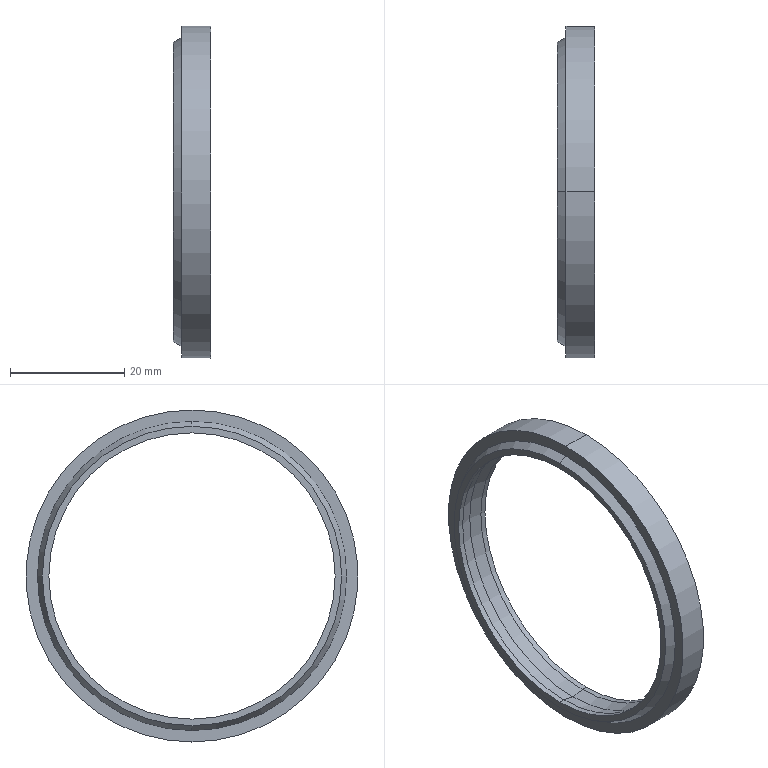Part | SolidWorks | features Revolution 2 | 1 solid | 22 faces | box 6.5 x 58 x 58 mm | volume 3242 mm3 | cone 10 | cylinder 6 | plane 4 | torus 2 | commonest cylinder face diameters 50 x4 58 x2
STEP:
#1=CARTESIAN_POINT('',(10.,0.,26.333));
#2=VERTEX_POINT('',#1);
#3=CARTESIAN_POINT('',(10.,0.,-26.333));
#4=VERTEX_POINT('',#3);
#5=CARTESIAN_POINT('',(10.,0.,0.));
#6=DIRECTION('',(-1.,0.,0.));
#7=DIRECTION('',(0.,0.,1.));
#8=AXIS2_PLACEMENT_3D('',#5,#6,#7);
#9=CIRCLE('',#8,26.333);
#10=EDGE_CURVE('',#2,#4,#9,.T.);
#11=ORIENTED_EDGE('',*,*,#10,.T.);
#12=CARTESIAN_POINT('',(7.47,0.,-26.853));
#13=VERTEX_POINT('',#12);
#14=CARTESIAN_POINT('',(10.,0.,-26.333));
#15=DIRECTION('',(-0.9795,0.,-0.2012));
#16=VECTOR('',#15,1000.);
#17=LINE('',#14,#16);
#18=EDGE_CURVE('',#4,#13,#17,.T.);
#19=ORIENTED_EDGE('',*,*,#18,.T.);
#20=CARTESIAN_POINT('',(7.47,0.,26.853));
#21=VERTEX_POINT('',#20);
#22=CARTESIAN_POINT('',(7.47,0.,0.));
#23=DIRECTION('',(-1.,0.,0.));
#24=DIRECTION('',(0.,0.,1.));
#25=AXIS2_PLACEMENT_3D('',#22,#23,#24);
#26=CIRCLE('',#25,26.853);
#27=EDGE_CURVE('',#21,#13,#26,.T.);
#28=ORIENTED_EDGE('',*,*,#27,.F.);
#29=CARTESIAN_POINT('',(10.,0.,26.333));
#30=DIRECTION('',(-0.9795,0.,0.2012));
#31=VECTOR('',#30,1000.);
#32=LINE('',#29,#31);
#33=EDGE_CURVE('',#2,#21,#32,.T.);
#34=ORIENTED_EDGE('',*,*,#33,.F.);
#35=EDGE_LOOP('',(#11,#19,#28,#34));
#36=FACE_OUTER_BOUND('',#35,.T.);
#37=CARTESIAN_POINT('',(10.,0.,0.));
#38=DIRECTION('',(-1.,0.,0.));
#39=DIRECTION('',(0.,0.,1.));
#40=AXIS2_PLACEMENT_3D('',#37,#38,#39);
#41=CONICAL_SURFACE('',#40,26.333,0.2026);
#42=ADVANCED_FACE('',(#36),#41,.T.);
#43=CARTESIAN_POINT('',(10.,0.,-25.));
#44=VERTEX_POINT('',#43);
#45=CARTESIAN_POINT('',(10.,0.,25.));
#46=VERTEX_POINT('',#45);
#47=CARTESIAN_POINT('',(10.,0.,0.));
#48=DIRECTION('',(-1.,0.,0.));
#49=DIRECTION('',(0.,0.,1.));
#50=AXIS2_PLACEMENT_3D('',#47,#48,#49);
#51=CIRCLE('',#50,25.);
#52=EDGE_CURVE('',#44,#46,#51,.T.);
#53=ORIENTED_EDGE('',*,*,#52,.F.);
#54=CARTESIAN_POINT('',(9.,0.,-25.));
#55=VERTEX_POINT('',#54);
#56=CARTESIAN_POINT('',(0.,0.,-25.));
#57=DIRECTION('',(-1.,0.,0.));
#58=VECTOR('',#57,1000.);
#59=LINE('',#56,#58);
#60=EDGE_CURVE('',#44,#55,#59,.T.);
#61=ORIENTED_EDGE('',*,*,#60,.T.);
#62=CARTESIAN_POINT('',(9.,0.,25.));
#63=VERTEX_POINT('',#62);
#64=CARTESIAN_POINT('',(9.,0.,0.));
#65=DIRECTION('',(-1.,0.,0.));
#66=DIRECTION('',(0.,0.,1.));
#67=AXIS2_PLACEMENT_3D('',#64,#65,#66);
#68=CIRCLE('',#67,25.);
#69=EDGE_CURVE('',#55,#63,#68,.T.);
#70=ORIENTED_EDGE('',*,*,#69,.T.);
#71=CARTESIAN_POINT('',(0.,0.,25.));
#72=DIRECTION('',(-1.,0.,0.));
#73=VECTOR('',#72,1000.);
#74=LINE('',#71,#73);
#75=EDGE_CURVE('',#46,#63,#74,.T.);
#76=ORIENTED_EDGE('',*,*,#75,.F.);
#77=EDGE_LOOP('',(#53,#61,#70,#76));
#78=FACE_OUTER_BOUND('',#77,.T.);
#79=CARTESIAN_POINT('',(0.,0.,0.));
#80=DIRECTION('',(-1.,0.,0.));
#81=DIRECTION('',(0.,0.,1.));
#82=AXIS2_PLACEMENT_3D('',#79,#80,#81);
#83=CYLINDRICAL_SURFACE('',#82,25.);
#84=ADVANCED_FACE('',(#78),#83,.F.);
#85=ORIENTED_EDGE('',*,*,#69,.F.);
#86=CARTESIAN_POINT('',(6.75,0.,-25.5));
#87=VERTEX_POINT('',#86);
#88=CARTESIAN_POINT('',(6.75,0.,-25.5));
#89=DIRECTION('',(-0.9762,0.,-0.2169));
#90=VECTOR('',#89,1000.);
#91=LINE('',#88,#90);
#92=EDGE_CURVE('',#55,#87,#91,.T.);
#93=ORIENTED_EDGE('',*,*,#92,.T.);
#94=CARTESIAN_POINT('',(6.75,0.,25.5));
#95=VERTEX_POINT('',#94);
#96=CARTESIAN_POINT('',(6.75,0.,0.));
#97=DIRECTION('',(-1.,0.,0.));
#98=DIRECTION('',(0.,0.,1.));
#99=AXIS2_PLACEMENT_3D('',#96,#97,#98);
#100=CIRCLE('',#99,25.5);
#101=EDGE_CURVE('',#87,#95,#100,.T.);
#102=ORIENTED_EDGE('',*,*,#101,.T.);
#103=CARTESIAN_POINT('',(6.75,0.,25.5));
#104=DIRECTION('',(-0.9762,0.,0.2169));
#105=VECTOR('',#104,1000.);
#106=LINE('',#103,#105);
#107=EDGE_CURVE('',#63,#95,#106,.T.);
#108=ORIENTED_EDGE('',*,*,#107,.F.);
#109=EDGE_LOOP('',(#85,#93,#102,#108));
#110=FACE_OUTER_BOUND('',#109,.T.);
#111=CARTESIAN_POINT('',(6.75,0.,0.));
#112=DIRECTION('',(-1.,0.,0.));
#113=DIRECTION('',(0.,0.,1.));
#114=AXIS2_PLACEMENT_3D('',#111,#112,#113);
#115=CONICAL_SURFACE('',#114,25.5,0.2187);
#116=ADVANCED_FACE('',(#110),#115,.F.);
#117=CARTESIAN_POINT('',(4.5,0.,-25.));
#118=VERTEX_POINT('',#117);
#119=CARTESIAN_POINT('',(4.5,0.,25.));
#120=VERTEX_POINT('',#119);
#121=CARTESIAN_POINT('',(4.5,0.,0.));
#122=DIRECTION('',(-1.,0.,0.));
#123=DIRECTION('',(0.,0.,1.));
#124=AXIS2_PLACEMENT_3D('',#121,#122,#123);
#125=CIRCLE('',#124,25.);
#126=EDGE_CURVE('',#118,#120,#125,.T.);
#127=ORIENTED_EDGE('',*,*,#126,.T.);
#128=CARTESIAN_POINT('',(4.5,0.,25.));
#129=DIRECTION('',(0.9762,0.,0.2169));
#130=VECTOR('',#129,1000.);
#131=LINE('',#128,#130);
#132=EDGE_CURVE('',#120,#95,#131,.T.);
#133=ORIENTED_EDGE('',*,*,#132,.T.);
#134=ORIENTED_EDGE('',*,*,#101,.F.);
#135=CARTESIAN_POINT('',(4.5,0.,-25.));
#136=DIRECTION('',(0.9762,0.,-0.2169));
#137=VECTOR('',#136,1000.);
#138=LINE('',#135,#137);
#139=EDGE_CURVE('',#118,#87,#138,.T.);
#140=ORIENTED_EDGE('',*,*,#139,.F.);
#141=EDGE_LOOP('',(#127,#133,#134,#140));
#142=FACE_OUTER_BOUND('',#141,.T.);
#143=CARTESIAN_POINT('',(4.5,0.,0.));
#144=DIRECTION('',(1.,0.,0.));
#145=DIRECTION('',(0.,0.,-1.));
#146=AXIS2_PLACEMENT_3D('',#143,#144,#145);
#147=CONICAL_SURFACE('',#146,25.,0.2187);
#148=ADVANCED_FACE('',(#142),#147,.F.);
#149=ORIENTED_EDGE('',*,*,#126,.F.);
#150=CARTESIAN_POINT('',(3.5,0.,-25.));
#151=VERTEX_POINT('',#150);
#152=CARTESIAN_POINT('',(0.,0.,-25.));
#153=DIRECTION('',(-1.,0.,0.));
#154=VECTOR('',#153,1000.);
#155=LINE('',#152,#154);
#156=EDGE_CURVE('',#118,#151,#155,.T.);
#157=ORIENTED_EDGE('',*,*,#156,.T.);
#158=CARTESIAN_POINT('',(3.5,0.,25.));
#159=VERTEX_POINT('',#158);
#160=CARTESIAN_POINT('',(3.5,0.,0.));
#161=DIRECTION('',(-1.,0.,0.));
#162=DIRECTION('',(0.,0.,1.));
#163=AXIS2_PLACEMENT_3D('',#160,#161,#162);
#164=CIRCLE('',#163,25.);
#165=EDGE_CURVE('',#151,#159,#164,.T.);
#166=ORIENTED_EDGE('',*,*,#165,.T.);
#167=CARTESIAN_POINT('',(0.,0.,25.));
#168=DIRECTION('',(-1.,0.,0.));
#169=VECTOR('',#168,1000.);
#170=LINE('',#167,#169);
#171=EDGE_CURVE('',#120,#159,#170,.T.);
#172=ORIENTED_EDGE('',*,*,#171,.F.);
#173=EDGE_LOOP('',(#149,#157,#166,#172));
#174=FACE_OUTER_BOUND('',#173,.T.);
#175=CARTESIAN_POINT('',(0.,0.,0.));
#176=DIRECTION('',(-1.,0.,0.));
#177=DIRECTION('',(0.,0.,1.));
#178=AXIS2_PLACEMENT_3D('',#175,#176,#177);
#179=CYLINDRICAL_SURFACE('',#178,25.);
#180=ADVANCED_FACE('',(#174),#179,.F.);
#181=CARTESIAN_POINT('',(3.5,0.,26.134));
#182=VERTEX_POINT('',#181);
#183=CARTESIAN_POINT('',(3.5,0.,-26.134));
#184=VERTEX_POINT('',#183);
#185=CARTESIAN_POINT('',(3.5,0.,0.));
#186=DIRECTION('',(-1.,0.,0.));
#187=DIRECTION('',(0.,0.,1.));
#188=AXIS2_PLACEMENT_3D('',#185,#186,#187);
#189=CIRCLE('',#188,26.134);
#190=EDGE_CURVE('',#182,#184,#189,.T.);
#191=ORIENTED_EDGE('',*,*,#190,.F.);
#192=CARTESIAN_POINT('',(5.,0.,27.));
#193=VERTEX_POINT('',#192);
#194=CARTESIAN_POINT('',(5.,0.,27.));
#195=DIRECTION('',(0.866,0.,0.5));
#196=VECTOR('',#195,1000.);
#197=LINE('',#194,#196);
#198=EDGE_CURVE('',#182,#193,#197,.T.);
#199=ORIENTED_EDGE('',*,*,#198,.T.);
#200=CARTESIAN_POINT('',(5.,0.,-27.));
#201=VERTEX_POINT('',#200);
#202=CARTESIAN_POINT('',(5.,0.,0.));
#203=DIRECTION('',(-1.,0.,0.));
#204=DIRECTION('',(0.,0.,1.));
#205=AXIS2_PLACEMENT_3D('',#202,#203,#204);
#206=CIRCLE('',#205,27.);
#207=EDGE_CURVE('',#193,#201,#206,.T.);
#208=ORIENTED_EDGE('',*,*,#207,.T.);
#209=CARTESIAN_POINT('',(5.,0.,-27.));
#210=DIRECTION('',(0.866,0.,-0.5));
#211=VECTOR('',#210,1000.);
#212=LINE('',#209,#211);
#213=EDGE_CURVE('',#184,#201,#212,.T.);
#214=ORIENTED_EDGE('',*,*,#213,.F.);
#215=EDGE_LOOP('',(#191,#199,#208,#214));
#216=FACE_OUTER_BOUND('',#215,.T.);
#217=CARTESIAN_POINT('',(5.,0.,0.));
#218=DIRECTION('',(1.,0.,0.));
#219=DIRECTION('',(0.,0.,-1.));
#220=AXIS2_PLACEMENT_3D('',#217,#218,#219);
#221=CONICAL_SURFACE('',#220,27.,0.5236);
#222=ADVANCED_FACE('',(#216),#221,.T.);
#223=CARTESIAN_POINT('',(10.,0.,29.));
#224=VERTEX_POINT('',#223);
#225=CARTESIAN_POINT('',(10.,0.,-29.));
#226=VERTEX_POINT('',#225);
#227=CARTESIAN_POINT('',(10.,0.,0.));
#228=DIRECTION('',(-1.,0.,0.));
#229=DIRECTION('',(0.,0.,1.));
#230=AXIS2_PLACEMENT_3D('',#227,#228,#229);
#231=CIRCLE('',#230,29.);
#232=EDGE_CURVE('',#224,#226,#231,.T.);
#233=ORIENTED_EDGE('',*,*,#232,.T.);
#234=CARTESIAN_POINT('',(5.,0.,-29.));
#235=VERTEX_POINT('',#234);
#236=CARTESIAN_POINT('',(0.,0.,-29.));
#237=DIRECTION('',(-1.,0.,0.));
#238=VECTOR('',#237,1000.);
#239=LINE('',#236,#238);
#240=EDGE_CURVE('',#226,#235,#239,.T.);
#241=ORIENTED_EDGE('',*,*,#240,.T.);
#242=CARTESIAN_POINT('',(5.,0.,29.));
#243=VERTEX_POINT('',#242);
#244=CARTESIAN_POINT('',(5.,0.,0.));
#245=DIRECTION('',(-1.,0.,0.));
#246=DIRECTION('',(0.,0.,1.));
#247=AXIS2_PLACEMENT_3D('',#244,#245,#246);
#248=CIRCLE('',#247,29.);
#249=EDGE_CURVE('',#243,#235,#248,.T.);
#250=ORIENTED_EDGE('',*,*,#249,.F.);
#251=CARTESIAN_POINT('',(0.,0.,29.));
#252=DIRECTION('',(-1.,0.,0.));
#253=VECTOR('',#252,1000.);
#254=LINE('',#251,#253);
#255=EDGE_CURVE('',#224,#243,#254,.T.);
#256=ORIENTED_EDGE('',*,*,#255,.F.);
#257=EDGE_LOOP('',(#233,#241,#250,#256));
#258=FACE_OUTER_BOUND('',#257,.T.);
#259=CARTESIAN_POINT('',(0.,0.,0.));
#260=DIRECTION('',(-1.,0.,0.));
#261=DIRECTION('',(0.,0.,1.));
#262=AXIS2_PLACEMENT_3D('',#259,#260,#261);
#263=CYLINDRICAL_SURFACE('',#262,29.);
#264=ADVANCED_FACE('',(#258),#263,.T.);
#265=CARTESIAN_POINT('',(7.47,0.,-27.147));
#266=VERTEX_POINT('',#265);
#267=CARTESIAN_POINT('',(7.47,0.,27.147));
#268=VERTEX_POINT('',#267);
#269=CARTESIAN_POINT('',(7.47,0.,0.));
#270=DIRECTION('',(-1.,0.,0.));
#271=DIRECTION('',(0.,0.,1.));
#272=AXIS2_PLACEMENT_3D('',#269,#270,#271);
#273=CIRCLE('',#272,27.147);
#274=EDGE_CURVE('',#266,#268,#273,.T.);
#275=ORIENTED_EDGE('',*,*,#274,.T.);
#276=CARTESIAN_POINT('',(10.,0.,27.667));
#277=VERTEX_POINT('',#276);
#278=CARTESIAN_POINT('',(10.,0.,27.667));
#279=DIRECTION('',(0.9795,0.,0.2012));
#280=VECTOR('',#279,1000.);
#281=LINE('',#278,#280);
#282=EDGE_CURVE('',#268,#277,#281,.T.);
#283=ORIENTED_EDGE('',*,*,#282,.T.);
#284=CARTESIAN_POINT('',(10.,0.,-27.667));
#285=VERTEX_POINT('',#284);
#286=CARTESIAN_POINT('',(10.,0.,0.));
#287=DIRECTION('',(-1.,0.,0.));
#288=DIRECTION('',(0.,0.,1.));
#289=AXIS2_PLACEMENT_3D('',#286,#287,#288);
#290=CIRCLE('',#289,27.667);
#291=EDGE_CURVE('',#285,#277,#290,.T.);
#292=ORIENTED_EDGE('',*,*,#291,.F.);
#293=CARTESIAN_POINT('',(10.,0.,-27.667));
#294=DIRECTION('',(0.9795,0.,-0.2012));
#295=VECTOR('',#294,1000.);
#296=LINE('',#293,#295);
#297=EDGE_CURVE('',#266,#285,#296,.T.);
#298=ORIENTED_EDGE('',*,*,#297,.F.);
#299=EDGE_LOOP('',(#275,#283,#292,#298));
#300=FACE_OUTER_BOUND('',#299,.T.);
#301=CARTESIAN_POINT('',(10.,0.,0.));
#302=DIRECTION('',(1.,0.,0.));
#303=DIRECTION('',(0.,0.,-1.));
#304=AXIS2_PLACEMENT_3D('',#301,#302,#303);
#305=CONICAL_SURFACE('',#304,27.667,0.2026);
#306=ADVANCED_FACE('',(#300),#305,.F.);
#307=ORIENTED_EDGE('',*,*,#274,.F.);
#308=CARTESIAN_POINT('',(7.5,0.,-27.));
#309=DIRECTION('',(0.,1.,0.));
#310=DIRECTION('',(-1.,0.,0.));
#311=AXIS2_PLACEMENT_3D('',#308,#309,#310);
#312=CIRCLE('',#311,0.15);
#313=EDGE_CURVE('',#266,#13,#312,.T.);
#314=ORIENTED_EDGE('',*,*,#313,.T.);
#315=CARTESIAN_POINT('',(7.47,0.,0.));
#316=DIRECTION('',(-1.,0.,0.));
#317=DIRECTION('',(0.,0.,1.));
#318=AXIS2_PLACEMENT_3D('',#315,#316,#317);
#319=CIRCLE('',#318,26.853);
#320=EDGE_CURVE('',#13,#21,#319,.T.);
#321=ORIENTED_EDGE('',*,*,#320,.T.);
#322=CARTESIAN_POINT('',(7.5,0.,27.));
#323=DIRECTION('',(0.,-1.,0.));
#324=DIRECTION('',(1.,0.,0.));
#325=AXIS2_PLACEMENT_3D('',#322,#323,#324);
#326=CIRCLE('',#325,0.15);
#327=EDGE_CURVE('',#268,#21,#326,.T.);
#328=ORIENTED_EDGE('',*,*,#327,.F.);
#329=EDGE_LOOP('',(#307,#314,#321,#328));
#330=FACE_OUTER_BOUND('',#329,.T.);
#331=CARTESIAN_POINT('',(7.5,0.,0.));
#332=DIRECTION('',(-1.,0.,0.));
#333=DIRECTION('',(0.,0.,1.));
#334=AXIS2_PLACEMENT_3D('',#331,#332,#333);
#335=TOROIDAL_SURFACE('',#334,27.,0.15);
#336=ADVANCED_FACE('',(#330),#335,.F.);
#337=ORIENTED_EDGE('',*,*,#313,.F.);
#338=CARTESIAN_POINT('',(7.47,0.,0.));
#339=DIRECTION('',(-1.,0.,0.));
#340=DIRECTION('',(0.,0.,1.));
#341=AXIS2_PLACEMENT_3D('',#338,#339,#340);
#342=CIRCLE('',#341,27.147);
#343=EDGE_CURVE('',#268,#266,#342,.T.);
#344=ORIENTED_EDGE('',*,*,#343,.F.);
#345=ORIENTED_EDGE('',*,*,#327,.T.);
#346=ORIENTED_EDGE('',*,*,#27,.T.);
#347=EDGE_LOOP('',(#337,#344,#345,#346));
#348=FACE_OUTER_BOUND('',#347,.T.);
#349=CARTESIAN_POINT('',(7.5,0.,0.));
#350=DIRECTION('',(-1.,0.,0.));
#351=DIRECTION('',(0.,0.,1.));
#352=AXIS2_PLACEMENT_3D('',#349,#350,#351);
#353=TOROIDAL_SURFACE('',#352,27.,0.15);
#354=ADVANCED_FACE('',(#348),#353,.F.);
#355=ORIENTED_EDGE('',*,*,#282,.F.);
#356=ORIENTED_EDGE('',*,*,#343,.T.);
#357=ORIENTED_EDGE('',*,*,#297,.T.);
#358=CARTESIAN_POINT('',(10.,0.,0.));
#359=DIRECTION('',(-1.,0.,0.));
#360=DIRECTION('',(0.,0.,1.));
#361=AXIS2_PLACEMENT_3D('',#358,#359,#360);
#362=CIRCLE('',#361,27.667);
#363=EDGE_CURVE('',#277,#285,#362,.T.);
#364=ORIENTED_EDGE('',*,*,#363,.F.);
#365=EDGE_LOOP('',(#355,#356,#357,#364));
#366=FACE_OUTER_BOUND('',#365,.T.);
#367=CARTESIAN_POINT('',(10.,0.,0.));
#368=DIRECTION('',(1.,0.,0.));
#369=DIRECTION('',(0.,0.,-1.));
#370=AXIS2_PLACEMENT_3D('',#367,#368,#369);
#371=CONICAL_SURFACE('',#370,27.667,0.2026);
#372=ADVANCED_FACE('',(#366),#371,.F.);
#373=ORIENTED_EDGE('',*,*,#291,.T.);
#374=ORIENTED_EDGE('',*,*,#363,.T.);
#375=EDGE_LOOP('',(#373,#374));
#376=FACE_BOUND('',#375,.T.);
#377=ORIENTED_EDGE('',*,*,#232,.F.);
#378=CARTESIAN_POINT('',(10.,0.,0.));
#379=DIRECTION('',(-1.,0.,0.));
#380=DIRECTION('',(0.,0.,1.));
#381=AXIS2_PLACEMENT_3D('',#378,#379,#380);
#382=CIRCLE('',#381,29.);
#383=EDGE_CURVE('',#226,#224,#382,.T.);
#384=ORIENTED_EDGE('',*,*,#383,.F.);
#385=EDGE_LOOP('',(#377,#384));
#386=FACE_OUTER_BOUND('',#385,.T.);
#387=CARTESIAN_POINT('',(10.,0.,0.));
#388=DIRECTION('',(1.,0.,0.));
#389=DIRECTION('',(0.,0.,-1.));
#390=AXIS2_PLACEMENT_3D('',#387,#388,#389);
#391=PLANE('',#390);
#392=ADVANCED_FACE('',(#376,#386),#391,.T.);
#393=ORIENTED_EDGE('',*,*,#240,.F.);
#394=ORIENTED_EDGE('',*,*,#383,.T.);
#395=ORIENTED_EDGE('',*,*,#255,.T.);
#396=CARTESIAN_POINT('',(5.,0.,0.));
#397=DIRECTION('',(-1.,0.,0.));
#398=DIRECTION('',(0.,0.,1.));
#399=AXIS2_PLACEMENT_3D('',#396,#397,#398);
#400=CIRCLE('',#399,29.);
#401=EDGE_CURVE('',#235,#243,#400,.T.);
#402=ORIENTED_EDGE('',*,*,#401,.F.);
#403=EDGE_LOOP('',(#393,#394,#395,#402));
#404=FACE_OUTER_BOUND('',#403,.T.);
#405=CARTESIAN_POINT('',(0.,0.,0.));
#406=DIRECTION('',(-1.,0.,0.));
#407=DIRECTION('',(0.,0.,1.));
#408=AXIS2_PLACEMENT_3D('',#405,#406,#407);
#409=CYLINDRICAL_SURFACE('',#408,29.);
#410=ADVANCED_FACE('',(#404),#409,.T.);
#411=CARTESIAN_POINT('',(5.,0.,0.));
#412=DIRECTION('',(-1.,0.,0.));
#413=DIRECTION('',(0.,0.,1.));
#414=AXIS2_PLACEMENT_3D('',#411,#412,#413);
#415=CIRCLE('',#414,27.);
#416=EDGE_CURVE('',#201,#193,#415,.T.);
#417=ORIENTED_EDGE('',*,*,#416,.F.);
#418=ORIENTED_EDGE('',*,*,#207,.F.);
#419=EDGE_LOOP('',(#417,#418));
#420=FACE_BOUND('',#419,.T.);
#421=ORIENTED_EDGE('',*,*,#249,.T.);
#422=ORIENTED_EDGE('',*,*,#401,.T.);
#423=EDGE_LOOP('',(#421,#422));
#424=FACE_OUTER_BOUND('',#423,.T.);
#425=CARTESIAN_POINT('',(5.,0.,0.));
#426=DIRECTION('',(1.,0.,0.));
#427=DIRECTION('',(0.,0.,-1.));
#428=AXIS2_PLACEMENT_3D('',#425,#426,#427);
#429=PLANE('',#428);
#430=ADVANCED_FACE('',(#420,#424),#429,.F.);
#431=ORIENTED_EDGE('',*,*,#198,.F.);
#432=CARTESIAN_POINT('',(3.5,0.,0.));
#433=DIRECTION('',(-1.,0.,0.));
#434=DIRECTION('',(0.,0.,1.));
#435=AXIS2_PLACEMENT_3D('',#432,#433,#434);
#436=CIRCLE('',#435,26.134);
#437=EDGE_CURVE('',#184,#182,#436,.T.);
#438=ORIENTED_EDGE('',*,*,#437,.F.);
#439=ORIENTED_EDGE('',*,*,#213,.T.);
#440=ORIENTED_EDGE('',*,*,#416,.T.);
#441=EDGE_LOOP('',(#431,#438,#439,#440));
#442=FACE_OUTER_BOUND('',#441,.T.);
#443=CARTESIAN_POINT('',(5.,0.,0.));
#444=DIRECTION('',(1.,0.,0.));
#445=DIRECTION('',(0.,0.,-1.));
#446=AXIS2_PLACEMENT_3D('',#443,#444,#445);
#447=CONICAL_SURFACE('',#446,27.,0.5236);
#448=ADVANCED_FACE('',(#442),#447,.T.);
#449=CARTESIAN_POINT('',(3.5,0.,0.));
#450=DIRECTION('',(-1.,0.,0.));
#451=DIRECTION('',(0.,0.,1.));
#452=AXIS2_PLACEMENT_3D('',#449,#450,#451);
#453=CIRCLE('',#452,25.);
#454=EDGE_CURVE('',#159,#151,#453,.T.);
#455=ORIENTED_EDGE('',*,*,#454,.F.);
#456=ORIENTED_EDGE('',*,*,#165,.F.);
#457=EDGE_LOOP('',(#455,#456));
#458=FACE_BOUND('',#457,.T.);
#459=ORIENTED_EDGE('',*,*,#437,.T.);
#460=ORIENTED_EDGE('',*,*,#190,.T.);
#461=EDGE_LOOP('',(#459,#460));
#462=FACE_OUTER_BOUND('',#461,.T.);
#463=CARTESIAN_POINT('',(3.5,0.,0.));
#464=DIRECTION('',(1.,0.,0.));
#465=DIRECTION('',(0.,0.,-1.));
#466=AXIS2_PLACEMENT_3D('',#463,#464,#465);
#467=PLANE('',#466);
#468=ADVANCED_FACE('',(#458,#462),#467,.F.);
#469=ORIENTED_EDGE('',*,*,#156,.F.);
#470=CARTESIAN_POINT('',(4.5,0.,0.));
#471=DIRECTION('',(-1.,0.,0.));
#472=DIRECTION('',(0.,0.,1.));
#473=AXIS2_PLACEMENT_3D('',#470,#471,#472);
#474=CIRCLE('',#473,25.);
#475=EDGE_CURVE('',#120,#118,#474,.T.);
#476=ORIENTED_EDGE('',*,*,#475,.F.);
#477=ORIENTED_EDGE('',*,*,#171,.T.);
#478=ORIENTED_EDGE('',*,*,#454,.T.);
#479=EDGE_LOOP('',(#469,#476,#477,#478));
#480=FACE_OUTER_BOUND('',#479,.T.);
#481=CARTESIAN_POINT('',(0.,0.,0.));
#482=DIRECTION('',(-1.,0.,0.));
#483=DIRECTION('',(0.,0.,1.));
#484=AXIS2_PLACEMENT_3D('',#481,#482,#483);
#485=CYLINDRICAL_SURFACE('',#484,25.);
#486=ADVANCED_FACE('',(#480),#485,.F.);
#487=ORIENTED_EDGE('',*,*,#132,.F.);
#488=ORIENTED_EDGE('',*,*,#475,.T.);
#489=ORIENTED_EDGE('',*,*,#139,.T.);
#490=CARTESIAN_POINT('',(6.75,0.,0.));
#491=DIRECTION('',(-1.,0.,0.));
#492=DIRECTION('',(0.,0.,1.));
#493=AXIS2_PLACEMENT_3D('',#490,#491,#492);
#494=CIRCLE('',#493,25.5);
#495=EDGE_CURVE('',#95,#87,#494,.T.);
#496=ORIENTED_EDGE('',*,*,#495,.F.);
#497=EDGE_LOOP('',(#487,#488,#489,#496));
#498=FACE_OUTER_BOUND('',#497,.T.);
#499=CARTESIAN_POINT('',(4.5,0.,0.));
#500=DIRECTION('',(1.,0.,0.));
#501=DIRECTION('',(0.,0.,-1.));
#502=AXIS2_PLACEMENT_3D('',#499,#500,#501);
#503=CONICAL_SURFACE('',#502,25.,0.2187);
#504=ADVANCED_FACE('',(#498),#503,.F.);
#505=ORIENTED_EDGE('',*,*,#92,.F.);
#506=CARTESIAN_POINT('',(9.,0.,0.));
#507=DIRECTION('',(-1.,0.,0.));
#508=DIRECTION('',(0.,0.,1.));
#509=AXIS2_PLACEMENT_3D('',#506,#507,#508);
#510=CIRCLE('',#509,25.);
#511=EDGE_CURVE('',#63,#55,#510,.T.);
#512=ORIENTED_EDGE('',*,*,#511,.F.);
#513=ORIENTED_EDGE('',*,*,#107,.T.);
#514=ORIENTED_EDGE('',*,*,#495,.T.);
#515=EDGE_LOOP('',(#505,#512,#513,#514));
#516=FACE_OUTER_BOUND('',#515,.T.);
#517=CARTESIAN_POINT('',(6.75,0.,0.));
#518=DIRECTION('',(-1.,0.,0.));
#519=DIRECTION('',(0.,0.,1.));
#520=AXIS2_PLACEMENT_3D('',#517,#518,#519);
#521=CONICAL_SURFACE('',#520,25.5,0.2187);
#522=ADVANCED_FACE('',(#516),#521,.F.);
#523=ORIENTED_EDGE('',*,*,#60,.F.);
#524=CARTESIAN_POINT('',(10.,0.,0.));
#525=DIRECTION('',(-1.,0.,0.));
#526=DIRECTION('',(0.,0.,1.));
#527=AXIS2_PLACEMENT_3D('',#524,#525,#526);
#528=CIRCLE('',#527,25.);
#529=EDGE_CURVE('',#46,#44,#528,.T.);
#530=ORIENTED_EDGE('',*,*,#529,.F.);
#531=ORIENTED_EDGE('',*,*,#75,.T.);
#532=ORIENTED_EDGE('',*,*,#511,.T.);
#533=EDGE_LOOP('',(#523,#530,#531,#532));
#534=FACE_OUTER_BOUND('',#533,.T.);
#535=CARTESIAN_POINT('',(0.,0.,0.));
#536=DIRECTION('',(-1.,0.,0.));
#537=DIRECTION('',(0.,0.,1.));
#538=AXIS2_PLACEMENT_3D('',#535,#536,#537);
#539=CYLINDRICAL_SURFACE('',#538,25.);
#540=ADVANCED_FACE('',(#534),#539,.F.);
#541=ORIENTED_EDGE('',*,*,#529,.T.);
#542=ORIENTED_EDGE('',*,*,#52,.T.);
#543=EDGE_LOOP('',(#541,#542));
#544=FACE_BOUND('',#543,.T.);
#545=ORIENTED_EDGE('',*,*,#10,.F.);
#546=CARTESIAN_POINT('',(10.,0.,0.));
#547=DIRECTION('',(-1.,0.,0.));
#548=DIRECTION('',(0.,0.,1.));
#549=AXIS2_PLACEMENT_3D('',#546,#547,#548);
#550=CIRCLE('',#549,26.333);
#551=EDGE_CURVE('',#4,#2,#550,.T.);
#552=ORIENTED_EDGE('',*,*,#551,.F.);
#553=EDGE_LOOP('',(#545,#552));
#554=FACE_OUTER_BOUND('',#553,.T.);
#555=CARTESIAN_POINT('',(10.,0.,0.));
#556=DIRECTION('',(1.,0.,0.));
#557=DIRECTION('',(0.,0.,-1.));
#558=AXIS2_PLACEMENT_3D('',#555,#556,#557);
#559=PLANE('',#558);
#560=ADVANCED_FACE('',(#544,#554),#559,.T.);
#561=ORIENTED_EDGE('',*,*,#18,.F.);
#562=ORIENTED_EDGE('',*,*,#551,.T.);
#563=ORIENTED_EDGE('',*,*,#33,.T.);
#564=ORIENTED_EDGE('',*,*,#320,.F.);
#565=EDGE_LOOP('',(#561,#562,#563,#564));
#566=FACE_OUTER_BOUND('',#565,.T.);
#567=CARTESIAN_POINT('',(10.,0.,0.));
#568=DIRECTION('',(-1.,0.,0.));
#569=DIRECTION('',(0.,0.,1.));
#570=AXIS2_PLACEMENT_3D('',#567,#568,#569);
#571=CONICAL_SURFACE('',#570,26.333,0.2026);
#572=ADVANCED_FACE('',(#566),#571,.T.);
#573=CLOSED_SHELL('',(#42,#84,#116,#148,#180,#222,#264,#306,#336,#354,#372,#392,#410,#430,#448,#468,#486,#504,#522,#540,#560,#572));
#574=MANIFOLD_SOLID_BREP('',#573);
#575=CARTESIAN_POINT('',(0.,0.,0.));
#576=DIRECTION('',(0.,0.,1.));
#577=DIRECTION('',(1.,0.,0.));
#578=AXIS2_PLACEMENT_3D('',#575,#576,#577);
#579=(LENGTH_UNIT()NAMED_UNIT(*)SI_UNIT(.MILLI.,.METRE.));
#580=UNCERTAINTY_MEASURE_WITH_UNIT(LENGTH_MEASURE(0.00001),#579,'','');
#581=(NAMED_UNIT(*)PLANE_ANGLE_UNIT()SI_UNIT($,.RADIAN.));
#582=(NAMED_UNIT(*)SI_UNIT($,.STERADIAN.)SOLID_ANGLE_UNIT());
#583=(GEOMETRIC_REPRESENTATION_CONTEXT(3)GLOBAL_UNCERTAINTY_ASSIGNED_CONTEXT((#580))GLOBAL_UNIT_ASSIGNED_CONTEXT((#579,#581,#582))REPRESENTATION_CONTEXT('',''));
#584=ADVANCED_BREP_SHAPE_REPRESENTATION('',(#574,#578),#583);